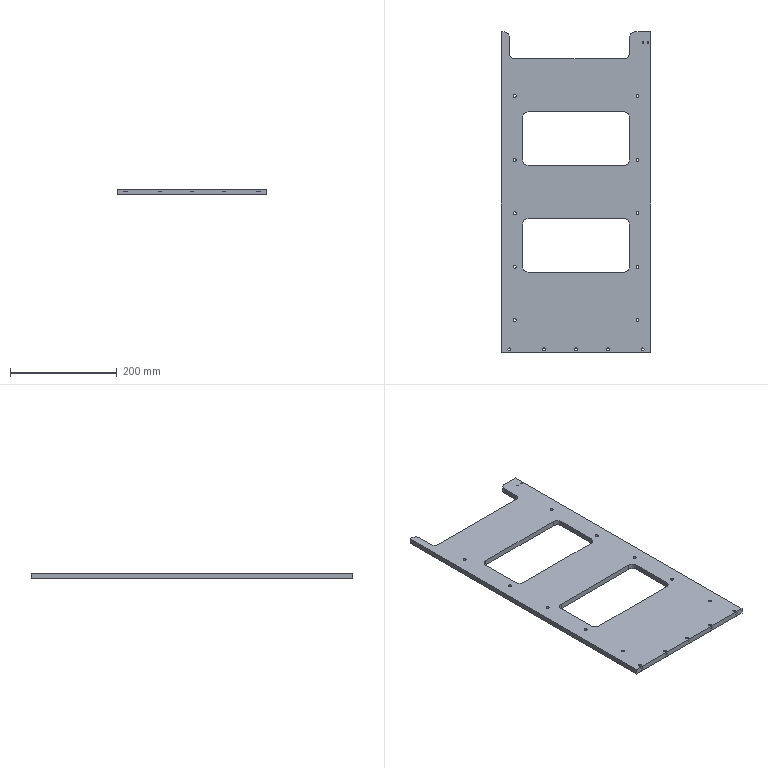Part | STEP file | PN_0033 | 1 solid | 109 faces | box 279.996 x 599.997 x 10 mm | volume 1160926 mm3 | cylinder 76 | plane 33 | commonest cylinder face diameters 5.5 x30 10 x20 20 x12 9.8 x10 2.5 x4